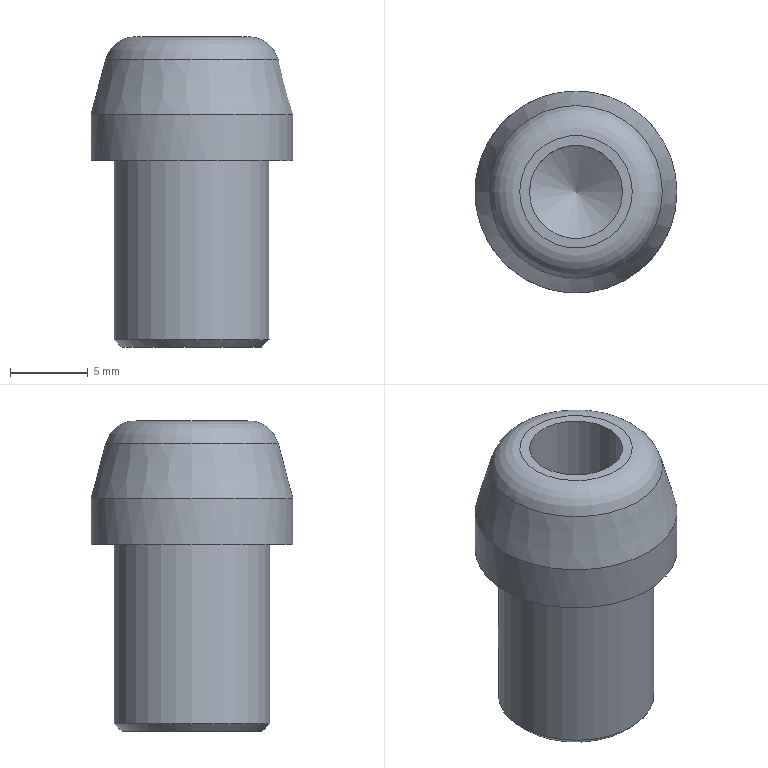Part | NX | features solid 2 | 1 solid | 10 faces | box 13 x 13 x 20 mm | volume 1559 mm3 | plane 3 | cylinder 3 | cone 3 | torus 1 | commonest cylinder face diameters 6 x1 10 x1 13 x1
STEP:
#1=CARTESIAN_POINT('',(126.967,-254.99,120.66));
#2=VERTEX_POINT('',#1);
#3=CARTESIAN_POINT('',(131.967,-254.99,120.66));
#4=DIRECTION('',(0.,0.,-1.));
#5=DIRECTION('',(-1.,0.,0.));
#6=AXIS2_PLACEMENT_3D('',#3,#4,#5);
#7=CIRCLE('',#6,5.);
#8=EDGE_CURVE('',#2,#2,#7,.T.);
#9=ORIENTED_EDGE('',*,*,#8,.F.);
#10=EDGE_LOOP('',(#9));
#11=FACE_BOUND('',#10,.T.);
#12=CARTESIAN_POINT('',(138.467,-254.99,120.66));
#13=VERTEX_POINT('',#12);
#14=CARTESIAN_POINT('',(131.967,-254.99,120.66));
#15=DIRECTION('',(0.,0.,1.));
#16=DIRECTION('',(1.,0.,0.));
#17=AXIS2_PLACEMENT_3D('',#14,#15,#16);
#18=CIRCLE('',#17,6.5);
#19=EDGE_CURVE('',#13,#13,#18,.T.);
#20=ORIENTED_EDGE('',*,*,#19,.F.);
#21=EDGE_LOOP('',(#20));
#22=FACE_BOUND('',#21,.T.);
#23=CARTESIAN_POINT('',(131.967,-254.99,120.66));
#24=DIRECTION('',(0.,0.,-1.));
#25=DIRECTION('',(-1.,0.,0.));
#26=AXIS2_PLACEMENT_3D('',#23,#24,#25);
#27=PLANE('',#26);
#28=ADVANCED_FACE('',(#11,#22),#27,.T.);
#29=CARTESIAN_POINT('',(125.467,-254.99,123.66));
#30=VERTEX_POINT('',#29);
#31=CARTESIAN_POINT('',(131.967,-254.99,123.66));
#32=DIRECTION('',(0.,0.,-1.));
#33=DIRECTION('',(-1.,0.,0.));
#34=AXIS2_PLACEMENT_3D('',#31,#32,#33);
#35=CIRCLE('',#34,6.5);
#36=EDGE_CURVE('',#30,#30,#35,.T.);
#37=ORIENTED_EDGE('',*,*,#36,.T.);
#38=EDGE_LOOP('',(#37));
#39=FACE_BOUND('',#38,.T.);
#40=ORIENTED_EDGE('',*,*,#19,.T.);
#41=EDGE_LOOP('',(#40));
#42=FACE_BOUND('',#41,.T.);
#43=CARTESIAN_POINT('',(131.967,-254.99,120.66));
#44=DIRECTION('',(0.,0.,1.));
#45=DIRECTION('',(1.,0.,0.));
#46=AXIS2_PLACEMENT_3D('',#43,#44,#45);
#47=CYLINDRICAL_SURFACE('',#46,6.5);
#48=ADVANCED_FACE('',(#39,#42),#47,.T.);
#49=CARTESIAN_POINT('',(126.409,-254.99,127.178));
#50=VERTEX_POINT('',#49);
#51=CARTESIAN_POINT('',(131.967,-254.99,127.178));
#52=DIRECTION('',(0.,0.,-1.));
#53=DIRECTION('',(-1.,0.,0.));
#54=AXIS2_PLACEMENT_3D('',#51,#52,#53);
#55=CIRCLE('',#54,5.557);
#56=EDGE_CURVE('',#50,#50,#55,.T.);
#57=ORIENTED_EDGE('',*,*,#56,.T.);
#58=EDGE_LOOP('',(#57));
#59=FACE_BOUND('',#58,.T.);
#60=ORIENTED_EDGE('',*,*,#36,.F.);
#61=EDGE_LOOP('',(#60));
#62=FACE_BOUND('',#61,.T.);
#63=CARTESIAN_POINT('',(131.967,-254.99,123.66));
#64=DIRECTION('',(0.,0.,-1.));
#65=DIRECTION('',(1.,0.,0.));
#66=AXIS2_PLACEMENT_3D('',#63,#64,#65);
#67=CONICAL_SURFACE('',#66,6.5,0.2618);
#68=ADVANCED_FACE('',(#59,#62),#67,.T.);
#69=CARTESIAN_POINT('',(128.967,-254.99,128.66));
#70=VERTEX_POINT('',#69);
#71=CARTESIAN_POINT('',(131.967,-254.99,128.66));
#72=DIRECTION('',(0.,0.,-1.));
#73=DIRECTION('',(-1.,0.,0.));
#74=AXIS2_PLACEMENT_3D('',#71,#72,#73);
#75=CIRCLE('',#74,3.);
#76=EDGE_CURVE('',#70,#70,#75,.T.);
#77=ORIENTED_EDGE('',*,*,#76,.T.);
#78=EDGE_LOOP('',(#77));
#79=FACE_BOUND('',#78,.T.);
#80=CARTESIAN_POINT('',(128.341,-254.99,128.66));
#81=VERTEX_POINT('',#80);
#82=CARTESIAN_POINT('',(131.967,-254.99,128.66));
#83=DIRECTION('',(0.,0.,-1.));
#84=DIRECTION('',(-1.,0.,0.));
#85=AXIS2_PLACEMENT_3D('',#82,#83,#84);
#86=CIRCLE('',#85,3.626);
#87=EDGE_CURVE('',#81,#81,#86,.F.);
#88=ORIENTED_EDGE('',*,*,#87,.T.);
#89=EDGE_LOOP('',(#88));
#90=FACE_BOUND('',#89,.T.);
#91=CARTESIAN_POINT('',(131.967,-254.99,128.66));
#92=DIRECTION('',(0.,0.,-1.));
#93=DIRECTION('',(-1.,0.,0.));
#94=AXIS2_PLACEMENT_3D('',#91,#92,#93);
#95=PLANE('',#94);
#96=ADVANCED_FACE('',(#79,#90),#95,.F.);
#97=CARTESIAN_POINT('',(127.467,-254.99,108.66));
#98=VERTEX_POINT('',#97);
#99=CARTESIAN_POINT('',(131.967,-254.99,108.66));
#100=DIRECTION('',(0.,0.,-1.));
#101=DIRECTION('',(-1.,0.,0.));
#102=AXIS2_PLACEMENT_3D('',#99,#100,#101);
#103=CIRCLE('',#102,4.5);
#104=EDGE_CURVE('',#98,#98,#103,.T.);
#105=ORIENTED_EDGE('',*,*,#104,.T.);
#106=EDGE_LOOP('',(#105));
#107=FACE_BOUND('',#106,.T.);
#108=CARTESIAN_POINT('',(131.967,-254.99,108.66));
#109=DIRECTION('',(0.,0.,-1.));
#110=DIRECTION('',(-1.,0.,0.));
#111=AXIS2_PLACEMENT_3D('',#108,#109,#110);
#112=PLANE('',#111);
#113=ADVANCED_FACE('',(#107),#112,.T.);
#114=CARTESIAN_POINT('',(126.967,-254.99,109.16));
#115=VERTEX_POINT('',#114);
#116=CARTESIAN_POINT('',(131.967,-254.99,109.16));
#117=DIRECTION('',(0.,0.,-1.));
#118=DIRECTION('',(-1.,0.,0.));
#119=AXIS2_PLACEMENT_3D('',#116,#117,#118);
#120=CIRCLE('',#119,5.);
#121=EDGE_CURVE('',#115,#115,#120,.F.);
#122=ORIENTED_EDGE('',*,*,#121,.T.);
#123=EDGE_LOOP('',(#122));
#124=FACE_BOUND('',#123,.T.);
#125=ORIENTED_EDGE('',*,*,#8,.T.);
#126=EDGE_LOOP('',(#125));
#127=FACE_BOUND('',#126,.T.);
#128=CARTESIAN_POINT('',(131.967,-254.99,120.66));
#129=DIRECTION('',(0.,0.,-1.));
#130=DIRECTION('',(-1.,0.,0.));
#131=AXIS2_PLACEMENT_3D('',#128,#129,#130);
#132=CYLINDRICAL_SURFACE('',#131,5.);
#133=ADVANCED_FACE('',(#124,#127),#132,.T.);
#134=ORIENTED_EDGE('',*,*,#121,.F.);
#135=EDGE_LOOP('',(#134));
#136=FACE_BOUND('',#135,.T.);
#137=ORIENTED_EDGE('',*,*,#104,.F.);
#138=EDGE_LOOP('',(#137));
#139=FACE_BOUND('',#138,.T.);
#140=CARTESIAN_POINT('',(131.967,-254.99,108.66));
#141=DIRECTION('',(0.,0.,1.));
#142=DIRECTION('',(1.,0.,0.));
#143=AXIS2_PLACEMENT_3D('',#140,#141,#142);
#144=CONICAL_SURFACE('',#143,4.5,0.7854);
#145=ADVANCED_FACE('',(#136,#139),#144,.T.);
#146=ORIENTED_EDGE('',*,*,#87,.F.);
#147=EDGE_LOOP('',(#146));
#148=FACE_BOUND('',#147,.T.);
#149=ORIENTED_EDGE('',*,*,#56,.F.);
#150=EDGE_LOOP('',(#149));
#151=FACE_BOUND('',#150,.T.);
#152=CARTESIAN_POINT('',(131.967,-254.99,126.66));
#153=DIRECTION('',(0.,0.,-1.));
#154=DIRECTION('',(-1.,0.,0.));
#155=AXIS2_PLACEMENT_3D('',#152,#153,#154);
#156=TOROIDAL_SURFACE('',#155,3.626,2.);
#157=ADVANCED_FACE('',(#148,#151),#156,.T.);
#158=CARTESIAN_POINT('',(128.967,-254.99,118.66));
#159=VERTEX_POINT('',#158);
#160=CARTESIAN_POINT('',(131.967,-254.99,118.66));
#161=DIRECTION('',(0.,0.,-1.));
#162=DIRECTION('',(-1.,0.,0.));
#163=AXIS2_PLACEMENT_3D('',#160,#161,#162);
#164=CIRCLE('',#163,3.);
#165=EDGE_CURVE('',#159,#159,#164,.T.);
#166=ORIENTED_EDGE('',*,*,#165,.F.);
#167=EDGE_LOOP('',(#166));
#168=FACE_BOUND('',#167,.T.);
#169=CARTESIAN_POINT('',(131.967,-254.99,116.857));
#170=VERTEX_POINT('',#169);
#171=VERTEX_LOOP('',#170);
#172=FACE_BOUND('',#171,.T.);
#173=CARTESIAN_POINT('',(131.967,-254.99,118.66));
#174=DIRECTION('',(0.,0.,1.));
#175=DIRECTION('',(1.,0.,0.));
#176=AXIS2_PLACEMENT_3D('',#173,#174,#175);
#177=CONICAL_SURFACE('',#176,3.,1.03);
#178=ADVANCED_FACE('',(#168,#172),#177,.F.);
#179=ORIENTED_EDGE('',*,*,#165,.T.);
#180=EDGE_LOOP('',(#179));
#181=FACE_BOUND('',#180,.T.);
#182=ORIENTED_EDGE('',*,*,#76,.F.);
#183=EDGE_LOOP('',(#182));
#184=FACE_BOUND('',#183,.T.);
#185=CARTESIAN_POINT('',(131.967,-254.99,128.66));
#186=DIRECTION('',(0.,0.,-1.));
#187=DIRECTION('',(-1.,0.,0.));
#188=AXIS2_PLACEMENT_3D('',#185,#186,#187);
#189=CYLINDRICAL_SURFACE('',#188,3.);
#190=ADVANCED_FACE('',(#181,#184),#189,.F.);
#191=CLOSED_SHELL('',(#28,#48,#68,#96,#113,#133,#145,#157,#178,#190));
#192=MANIFOLD_SOLID_BREP('',#191);
#193=(LENGTH_UNIT()NAMED_UNIT(*)SI_UNIT(.MILLI.,.METRE.));
#194=UNCERTAINTY_MEASURE_WITH_UNIT(LENGTH_MEASURE(0.00001),#193,'','');
#195=(NAMED_UNIT(*)PLANE_ANGLE_UNIT()SI_UNIT($,.RADIAN.));
#196=(NAMED_UNIT(*)SI_UNIT($,.STERADIAN.)SOLID_ANGLE_UNIT());
#197=(GEOMETRIC_REPRESENTATION_CONTEXT(3)GLOBAL_UNCERTAINTY_ASSIGNED_CONTEXT((#194))GLOBAL_UNIT_ASSIGNED_CONTEXT((#193,#195,#196))REPRESENTATION_CONTEXT('',''));
#198=ADVANCED_BREP_SHAPE_REPRESENTATION('',(#192),#197);